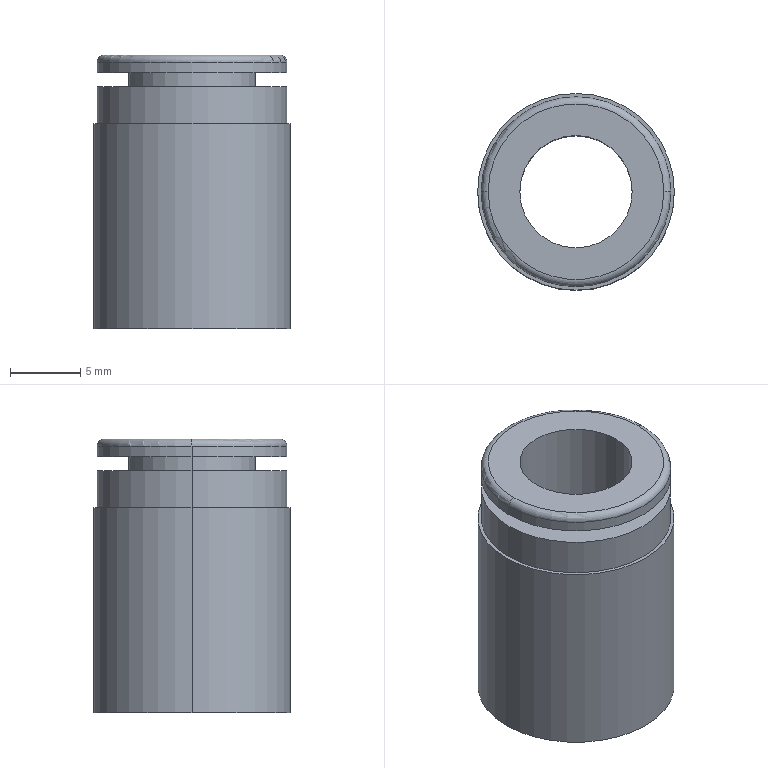Part | STEP file | SS5V1-16S3AD-08B-N1_SV Fittings | 1 solid | 17 faces | box 14 x 14 x 19.5 mm | volume 1887 mm3 | cylinder 10 | plane 5 | torus 2 | commonest cylinder face diameters 13.5 x4 8 x2 9 x2 14 x2
STEP:
#1=CARTESIAN_POINT('',(0.,0.,0.));
#2=DIRECTION('',(0.,0.,1.));
#3=DIRECTION('',(1.,0.,0.));
#4=AXIS2_PLACEMENT_3D('',#1,#2,#3);
#5=CARTESIAN_POINT('',(-6.75,0.,19.));
#6=VERTEX_POINT('',#5);
#7=CARTESIAN_POINT('',(6.75,0.,19.));
#8=VERTEX_POINT('',#7);
#9=CARTESIAN_POINT('',(0.,0.,19.));
#10=DIRECTION('',(0.,0.,-1.));
#11=DIRECTION('',(1.,0.,0.));
#12=AXIS2_PLACEMENT_3D('',#9,#10,#11);
#13=CIRCLE('',#12,6.75);
#14=CARTESIAN_POINT('',(0.,0.,19.));
#15=DIRECTION('',(0.,0.,1.));
#16=DIRECTION('',(1.,0.,0.));
#17=AXIS2_PLACEMENT_3D('',#14,#15,#16);
#18=TOROIDAL_SURFACE('',#17,6.25,0.5);
#19=CARTESIAN_POINT('',(6.283,0.));
#20=DIRECTION('',(-1.,0.));
#21=VECTOR('',#20,1.);
#22=LINE('',#19,#21);
#23=(GEOMETRIC_REPRESENTATION_CONTEXT(2)PARAMETRIC_REPRESENTATION_CONTEXT()REPRESENTATION_CONTEXT('',''));
#24=DEFINITIONAL_REPRESENTATION('',(#22),#23);
#25=PCURVE('',#18,#24);
#26=CARTESIAN_POINT('',(0.,0.,19.5));
#27=DIRECTION('',(0.,0.,-1.));
#28=DIRECTION('',(-1.,0.,0.));
#29=AXIS2_PLACEMENT_3D('',#26,#27,#28);
#30=CYLINDRICAL_SURFACE('',#29,6.75);
#31=CARTESIAN_POINT('',(-3.142,0.5));
#32=DIRECTION('',(1.,0.));
#33=VECTOR('',#32,1.);
#34=LINE('',#31,#33);
#35=(GEOMETRIC_REPRESENTATION_CONTEXT(2)PARAMETRIC_REPRESENTATION_CONTEXT()REPRESENTATION_CONTEXT('',''));
#36=DEFINITIONAL_REPRESENTATION('',(#34),#35);
#37=PCURVE('',#30,#36);
#38=SURFACE_CURVE('',#13,(#25,#37),.PCURVE_S1.);
#39=EDGE_CURVE('',#6,#8,#38,.T.);
#40=ORIENTED_EDGE('',*,*,#39,.F.);
#41=CARTESIAN_POINT('',(-6.25,0.,19.5));
#42=VERTEX_POINT('',#41);
#43=CARTESIAN_POINT('',(-6.25,0.,19.));
#44=DIRECTION('',(0.,1.,0.));
#45=DIRECTION('',(-1.,0.,0.));
#46=AXIS2_PLACEMENT_3D('',#43,#44,#45);
#47=CIRCLE('',#46,0.5);
#48=CARTESIAN_POINT('',(3.142,0.));
#49=DIRECTION('',(0.,1.));
#50=VECTOR('',#49,1.);
#51=LINE('',#48,#50);
#52=(GEOMETRIC_REPRESENTATION_CONTEXT(2)PARAMETRIC_REPRESENTATION_CONTEXT()REPRESENTATION_CONTEXT('',''));
#53=DEFINITIONAL_REPRESENTATION('',(#51),#52);
#54=PCURVE('',#18,#53);
#55=CARTESIAN_POINT('',(0.,0.,19.));
#56=DIRECTION('',(0.,0.,1.));
#57=DIRECTION('',(1.,0.,0.));
#58=AXIS2_PLACEMENT_3D('',#55,#56,#57);
#59=TOROIDAL_SURFACE('',#58,6.25,0.5);
#60=CARTESIAN_POINT('',(3.142,0.));
#61=DIRECTION('',(0.,1.));
#62=VECTOR('',#61,1.);
#63=LINE('',#60,#62);
#64=(GEOMETRIC_REPRESENTATION_CONTEXT(2)PARAMETRIC_REPRESENTATION_CONTEXT()REPRESENTATION_CONTEXT('',''));
#65=DEFINITIONAL_REPRESENTATION('',(#63),#64);
#66=PCURVE('',#59,#65);
#67=SURFACE_CURVE('',#47,(#54,#66),.PCURVE_S1.);
#68=EDGE_CURVE('',#6,#42,#67,.T.);
#69=ORIENTED_EDGE('',*,*,#68,.T.);
#70=CARTESIAN_POINT('',(6.25,0.,19.5));
#71=VERTEX_POINT('',#70);
#72=CARTESIAN_POINT('',(0.,0.,19.5));
#73=DIRECTION('',(0.,0.,1.));
#74=DIRECTION('',(1.,0.,0.));
#75=AXIS2_PLACEMENT_3D('',#72,#73,#74);
#76=CIRCLE('',#75,6.25);
#77=CARTESIAN_POINT('',(0.,1.571));
#78=DIRECTION('',(1.,0.));
#79=VECTOR('',#78,1.);
#80=LINE('',#77,#79);
#81=(GEOMETRIC_REPRESENTATION_CONTEXT(2)PARAMETRIC_REPRESENTATION_CONTEXT()REPRESENTATION_CONTEXT('',''));
#82=DEFINITIONAL_REPRESENTATION('',(#80),#81);
#83=PCURVE('',#18,#82);
#84=CARTESIAN_POINT('',(0.,0.,19.5));
#85=DIRECTION('',(0.,0.,1.));
#86=DIRECTION('',(1.,0.,0.));
#87=AXIS2_PLACEMENT_3D('',#84,#85,#86);
#88=PLANE('',#87);
#89=CARTESIAN_POINT('',(0.,0.));
#90=DIRECTION('',(1.,0.));
#91=AXIS2_PLACEMENT_2D('',#89,#90);
#92=CIRCLE('',#91,6.25);
#93=(GEOMETRIC_REPRESENTATION_CONTEXT(2)PARAMETRIC_REPRESENTATION_CONTEXT()REPRESENTATION_CONTEXT('',''));
#94=DEFINITIONAL_REPRESENTATION('',(#92),#93);
#95=PCURVE('',#88,#94);
#96=SURFACE_CURVE('',#76,(#83,#95),.PCURVE_S1.);
#97=EDGE_CURVE('',#71,#42,#96,.T.);
#98=ORIENTED_EDGE('',*,*,#97,.F.);
#99=CARTESIAN_POINT('',(6.25,0.,19.));
#100=DIRECTION('',(0.,-1.,0.));
#101=DIRECTION('',(0.,0.,-1.));
#102=AXIS2_PLACEMENT_3D('',#99,#100,#101);
#103=CIRCLE('',#102,0.5);
#104=CARTESIAN_POINT('',(0.,-1.571));
#105=DIRECTION('',(0.,1.));
#106=VECTOR('',#105,1.);
#107=LINE('',#104,#106);
#108=(GEOMETRIC_REPRESENTATION_CONTEXT(2)PARAMETRIC_REPRESENTATION_CONTEXT()REPRESENTATION_CONTEXT('',''));
#109=DEFINITIONAL_REPRESENTATION('',(#107),#108);
#110=PCURVE('',#18,#109);
#111=CARTESIAN_POINT('',(6.283,-1.571));
#112=DIRECTION('',(0.,1.));
#113=VECTOR('',#112,1.);
#114=LINE('',#111,#113);
#115=(GEOMETRIC_REPRESENTATION_CONTEXT(2)PARAMETRIC_REPRESENTATION_CONTEXT()REPRESENTATION_CONTEXT('',''));
#116=DEFINITIONAL_REPRESENTATION('',(#114),#115);
#117=PCURVE('',#59,#116);
#118=SURFACE_CURVE('',#103,(#110,#117),.PCURVE_S1.);
#119=EDGE_CURVE('',#8,#71,#118,.T.);
#120=ORIENTED_EDGE('',*,*,#119,.F.);
#121=EDGE_LOOP('',(#40,#69,#98,#120));
#122=FACE_BOUND('',#121,.T.);
#123=ADVANCED_FACE('',(#122),#18,.T.);
#124=ORIENTED_EDGE('',*,*,#39,.T.);
#125=CARTESIAN_POINT('',(6.75,0.,18.25));
#126=VERTEX_POINT('',#125);
#127=CARTESIAN_POINT('',(6.75,0.,19.5));
#128=DIRECTION('',(0.,0.,-1.));
#129=VECTOR('',#128,1.);
#130=LINE('',#127,#129);
#131=CARTESIAN_POINT('',(3.142,0.));
#132=DIRECTION('',(0.,1.));
#133=VECTOR('',#132,1.);
#134=LINE('',#131,#133);
#135=(GEOMETRIC_REPRESENTATION_CONTEXT(2)PARAMETRIC_REPRESENTATION_CONTEXT()REPRESENTATION_CONTEXT('',''));
#136=DEFINITIONAL_REPRESENTATION('',(#134),#135);
#137=PCURVE('',#30,#136);
#138=CARTESIAN_POINT('',(0.,0.,19.5));
#139=DIRECTION('',(0.,0.,-1.));
#140=DIRECTION('',(-1.,0.,0.));
#141=AXIS2_PLACEMENT_3D('',#138,#139,#140);
#142=CYLINDRICAL_SURFACE('',#141,6.75);
#143=CARTESIAN_POINT('',(3.142,0.));
#144=DIRECTION('',(0.,1.));
#145=VECTOR('',#144,1.);
#146=LINE('',#143,#145);
#147=(GEOMETRIC_REPRESENTATION_CONTEXT(2)PARAMETRIC_REPRESENTATION_CONTEXT()REPRESENTATION_CONTEXT('',''));
#148=DEFINITIONAL_REPRESENTATION('',(#146),#147);
#149=PCURVE('',#142,#148);
#150=SURFACE_CURVE('',#130,(#137,#149),.PCURVE_S1.);
#151=EDGE_CURVE('',#8,#126,#150,.T.);
#152=ORIENTED_EDGE('',*,*,#151,.T.);
#153=CARTESIAN_POINT('',(-6.75,0.,18.25));
#154=VERTEX_POINT('',#153);
#155=CARTESIAN_POINT('',(0.,0.,18.25));
#156=DIRECTION('',(0.,0.,1.));
#157=DIRECTION('',(1.,0.,0.));
#158=AXIS2_PLACEMENT_3D('',#155,#156,#157);
#159=CIRCLE('',#158,6.75);
#160=CARTESIAN_POINT('',(3.142,1.25));
#161=DIRECTION('',(-1.,0.));
#162=VECTOR('',#161,1.);
#163=LINE('',#160,#162);
#164=(GEOMETRIC_REPRESENTATION_CONTEXT(2)PARAMETRIC_REPRESENTATION_CONTEXT()REPRESENTATION_CONTEXT('',''));
#165=DEFINITIONAL_REPRESENTATION('',(#163),#164);
#166=PCURVE('',#30,#165);
#167=CARTESIAN_POINT('',(0.,0.,18.25));
#168=DIRECTION('',(0.,0.,1.));
#169=DIRECTION('',(1.,0.,0.));
#170=AXIS2_PLACEMENT_3D('',#167,#168,#169);
#171=PLANE('',#170);
#172=CARTESIAN_POINT('',(0.,0.));
#173=DIRECTION('',(1.,0.));
#174=AXIS2_PLACEMENT_2D('',#172,#173);
#175=CIRCLE('',#174,6.75);
#176=(GEOMETRIC_REPRESENTATION_CONTEXT(2)PARAMETRIC_REPRESENTATION_CONTEXT()REPRESENTATION_CONTEXT('',''));
#177=DEFINITIONAL_REPRESENTATION('',(#175),#176);
#178=PCURVE('',#171,#177);
#179=SURFACE_CURVE('',#159,(#166,#178),.PCURVE_S1.);
#180=EDGE_CURVE('',#126,#154,#179,.T.);
#181=ORIENTED_EDGE('',*,*,#180,.T.);
#182=CARTESIAN_POINT('',(-6.75,0.,19.5));
#183=DIRECTION('',(0.,0.,-1.));
#184=VECTOR('',#183,1.);
#185=LINE('',#182,#184);
#186=CARTESIAN_POINT('',(0.,0.));
#187=DIRECTION('',(0.,1.));
#188=VECTOR('',#187,1.);
#189=LINE('',#186,#188);
#190=(GEOMETRIC_REPRESENTATION_CONTEXT(2)PARAMETRIC_REPRESENTATION_CONTEXT()REPRESENTATION_CONTEXT('',''));
#191=DEFINITIONAL_REPRESENTATION('',(#189),#190);
#192=PCURVE('',#30,#191);
#193=CARTESIAN_POINT('',(6.283,0.));
#194=DIRECTION('',(0.,1.));
#195=VECTOR('',#194,1.);
#196=LINE('',#193,#195);
#197=(GEOMETRIC_REPRESENTATION_CONTEXT(2)PARAMETRIC_REPRESENTATION_CONTEXT()REPRESENTATION_CONTEXT('',''));
#198=DEFINITIONAL_REPRESENTATION('',(#196),#197);
#199=PCURVE('',#142,#198);
#200=SURFACE_CURVE('',#185,(#192,#199),.PCURVE_S1.);
#201=EDGE_CURVE('',#6,#154,#200,.T.);
#202=ORIENTED_EDGE('',*,*,#201,.F.);
#203=EDGE_LOOP('',(#124,#152,#181,#202));
#204=FACE_BOUND('',#203,.T.);
#205=ADVANCED_FACE('',(#204),#30,.T.);
#206=CARTESIAN_POINT('',(4.5,0.,18.25));
#207=VERTEX_POINT('',#206);
#208=CARTESIAN_POINT('',(-4.5,0.,18.25));
#209=VERTEX_POINT('',#208);
#210=CARTESIAN_POINT('',(0.,0.,18.25));
#211=DIRECTION('',(0.,0.,1.));
#212=DIRECTION('',(1.,0.,0.));
#213=AXIS2_PLACEMENT_3D('',#210,#211,#212);
#214=CIRCLE('',#213,4.5);
#215=CARTESIAN_POINT('',(0.,0.,18.25));
#216=DIRECTION('',(0.,0.,-1.));
#217=DIRECTION('',(-1.,0.,0.));
#218=AXIS2_PLACEMENT_3D('',#215,#216,#217);
#219=CYLINDRICAL_SURFACE('',#218,4.5);
#220=CARTESIAN_POINT('',(3.142,0.));
#221=DIRECTION('',(-1.,0.));
#222=VECTOR('',#221,1.);
#223=LINE('',#220,#222);
#224=(GEOMETRIC_REPRESENTATION_CONTEXT(2)PARAMETRIC_REPRESENTATION_CONTEXT()REPRESENTATION_CONTEXT('',''));
#225=DEFINITIONAL_REPRESENTATION('',(#223),#224);
#226=PCURVE('',#219,#225);
#227=CARTESIAN_POINT('',(0.,0.));
#228=DIRECTION('',(1.,0.));
#229=AXIS2_PLACEMENT_2D('',#227,#228);
#230=CIRCLE('',#229,4.5);
#231=(GEOMETRIC_REPRESENTATION_CONTEXT(2)PARAMETRIC_REPRESENTATION_CONTEXT()REPRESENTATION_CONTEXT('',''));
#232=DEFINITIONAL_REPRESENTATION('',(#230),#231);
#233=PCURVE('',#171,#232);
#234=SURFACE_CURVE('',#214,(#226,#233),.PCURVE_S1.);
#235=EDGE_CURVE('',#207,#209,#234,.T.);
#236=ORIENTED_EDGE('',*,*,#235,.F.);
#237=CARTESIAN_POINT('',(4.5,0.,17.25));
#238=VERTEX_POINT('',#237);
#239=CARTESIAN_POINT('',(4.5,0.,18.25));
#240=DIRECTION('',(0.,0.,-1.));
#241=VECTOR('',#240,1.);
#242=LINE('',#239,#241);
#243=CARTESIAN_POINT('',(3.142,0.));
#244=DIRECTION('',(0.,1.));
#245=VECTOR('',#244,1.);
#246=LINE('',#243,#245);
#247=(GEOMETRIC_REPRESENTATION_CONTEXT(2)PARAMETRIC_REPRESENTATION_CONTEXT()REPRESENTATION_CONTEXT('',''));
#248=DEFINITIONAL_REPRESENTATION('',(#246),#247);
#249=PCURVE('',#219,#248);
#250=CARTESIAN_POINT('',(0.,0.,18.25));
#251=DIRECTION('',(0.,0.,-1.));
#252=DIRECTION('',(-1.,0.,0.));
#253=AXIS2_PLACEMENT_3D('',#250,#251,#252);
#254=CYLINDRICAL_SURFACE('',#253,4.5);
#255=CARTESIAN_POINT('',(3.142,0.));
#256=DIRECTION('',(0.,1.));
#257=VECTOR('',#256,1.);
#258=LINE('',#255,#257);
#259=(GEOMETRIC_REPRESENTATION_CONTEXT(2)PARAMETRIC_REPRESENTATION_CONTEXT()REPRESENTATION_CONTEXT('',''));
#260=DEFINITIONAL_REPRESENTATION('',(#258),#259);
#261=PCURVE('',#254,#260);
#262=SURFACE_CURVE('',#242,(#249,#261),.PCURVE_S1.);
#263=EDGE_CURVE('',#207,#238,#262,.T.);
#264=ORIENTED_EDGE('',*,*,#263,.T.);
#265=CARTESIAN_POINT('',(-4.5,0.,17.25));
#266=VERTEX_POINT('',#265);
#267=CARTESIAN_POINT('',(0.,0.,17.25));
#268=DIRECTION('',(0.,0.,1.));
#269=DIRECTION('',(1.,0.,0.));
#270=AXIS2_PLACEMENT_3D('',#267,#268,#269);
#271=CIRCLE('',#270,4.5);
#272=CARTESIAN_POINT('',(3.142,1.));
#273=DIRECTION('',(-1.,0.));
#274=VECTOR('',#273,1.);
#275=LINE('',#272,#274);
#276=(GEOMETRIC_REPRESENTATION_CONTEXT(2)PARAMETRIC_REPRESENTATION_CONTEXT()REPRESENTATION_CONTEXT('',''));
#277=DEFINITIONAL_REPRESENTATION('',(#275),#276);
#278=PCURVE('',#219,#277);
#279=CARTESIAN_POINT('',(0.,0.,17.25));
#280=DIRECTION('',(0.,0.,1.));
#281=DIRECTION('',(1.,0.,0.));
#282=AXIS2_PLACEMENT_3D('',#279,#280,#281);
#283=PLANE('',#282);
#284=CARTESIAN_POINT('',(0.,0.));
#285=DIRECTION('',(1.,0.));
#286=AXIS2_PLACEMENT_2D('',#284,#285);
#287=CIRCLE('',#286,4.5);
#288=(GEOMETRIC_REPRESENTATION_CONTEXT(2)PARAMETRIC_REPRESENTATION_CONTEXT()REPRESENTATION_CONTEXT('',''));
#289=DEFINITIONAL_REPRESENTATION('',(#287),#288);
#290=PCURVE('',#283,#289);
#291=SURFACE_CURVE('',#271,(#278,#290),.PCURVE_S1.);
#292=EDGE_CURVE('',#238,#266,#291,.T.);
#293=ORIENTED_EDGE('',*,*,#292,.T.);
#294=CARTESIAN_POINT('',(-4.5,0.,18.25));
#295=DIRECTION('',(0.,0.,-1.));
#296=VECTOR('',#295,1.);
#297=LINE('',#294,#296);
#298=CARTESIAN_POINT('',(0.,0.));
#299=DIRECTION('',(0.,1.));
#300=VECTOR('',#299,1.);
#301=LINE('',#298,#300);
#302=(GEOMETRIC_REPRESENTATION_CONTEXT(2)PARAMETRIC_REPRESENTATION_CONTEXT()REPRESENTATION_CONTEXT('',''));
#303=DEFINITIONAL_REPRESENTATION('',(#301),#302);
#304=PCURVE('',#219,#303);
#305=CARTESIAN_POINT('',(6.283,0.));
#306=DIRECTION('',(0.,1.));
#307=VECTOR('',#306,1.);
#308=LINE('',#305,#307);
#309=(GEOMETRIC_REPRESENTATION_CONTEXT(2)PARAMETRIC_REPRESENTATION_CONTEXT()REPRESENTATION_CONTEXT('',''));
#310=DEFINITIONAL_REPRESENTATION('',(#308),#309);
#311=PCURVE('',#254,#310);
#312=SURFACE_CURVE('',#297,(#304,#311),.PCURVE_S1.);
#313=EDGE_CURVE('',#209,#266,#312,.T.);
#314=ORIENTED_EDGE('',*,*,#313,.F.);
#315=EDGE_LOOP('',(#236,#264,#293,#314));
#316=FACE_BOUND('',#315,.T.);
#317=ADVANCED_FACE('',(#316),#219,.T.);
#318=CARTESIAN_POINT('',(6.75,0.,17.25));
#319=VERTEX_POINT('',#318);
#320=CARTESIAN_POINT('',(-6.75,0.,17.25));
#321=VERTEX_POINT('',#320);
#322=CARTESIAN_POINT('',(0.,0.,17.25));
#323=DIRECTION('',(0.,0.,1.));
#324=DIRECTION('',(1.,0.,0.));
#325=AXIS2_PLACEMENT_3D('',#322,#323,#324);
#326=CIRCLE('',#325,6.75);
#327=CARTESIAN_POINT('',(0.,0.,17.25));
#328=DIRECTION('',(0.,0.,-1.));
#329=DIRECTION('',(-1.,0.,0.));
#330=AXIS2_PLACEMENT_3D('',#327,#328,#329);
#331=CYLINDRICAL_SURFACE('',#330,6.75);
#332=CARTESIAN_POINT('',(3.142,0.));
#333=DIRECTION('',(-1.,0.));
#334=VECTOR('',#333,1.);
#335=LINE('',#332,#334);
#336=(GEOMETRIC_REPRESENTATION_CONTEXT(2)PARAMETRIC_REPRESENTATION_CONTEXT()REPRESENTATION_CONTEXT('',''));
#337=DEFINITIONAL_REPRESENTATION('',(#335),#336);
#338=PCURVE('',#331,#337);
#339=CARTESIAN_POINT('',(0.,0.));
#340=DIRECTION('',(1.,0.));
#341=AXIS2_PLACEMENT_2D('',#339,#340);
#342=CIRCLE('',#341,6.75);
#343=(GEOMETRIC_REPRESENTATION_CONTEXT(2)PARAMETRIC_REPRESENTATION_CONTEXT()REPRESENTATION_CONTEXT('',''));
#344=DEFINITIONAL_REPRESENTATION('',(#342),#343);
#345=PCURVE('',#283,#344);
#346=SURFACE_CURVE('',#326,(#338,#345),.PCURVE_S1.);
#347=EDGE_CURVE('',#319,#321,#346,.T.);
#348=ORIENTED_EDGE('',*,*,#347,.F.);
#349=CARTESIAN_POINT('',(6.75,0.,14.6));
#350=VERTEX_POINT('',#349);
#351=CARTESIAN_POINT('',(6.75,0.,17.25));
#352=DIRECTION('',(0.,0.,-1.));
#353=VECTOR('',#352,1.);
#354=LINE('',#351,#353);
#355=CARTESIAN_POINT('',(3.142,0.));
#356=DIRECTION('',(0.,1.));
#357=VECTOR('',#356,1.);
#358=LINE('',#355,#357);
#359=(GEOMETRIC_REPRESENTATION_CONTEXT(2)PARAMETRIC_REPRESENTATION_CONTEXT()REPRESENTATION_CONTEXT('',''));
#360=DEFINITIONAL_REPRESENTATION('',(#358),#359);
#361=PCURVE('',#331,#360);
#362=CARTESIAN_POINT('',(0.,0.,17.25));
#363=DIRECTION('',(0.,0.,-1.));
#364=DIRECTION('',(-1.,0.,0.));
#365=AXIS2_PLACEMENT_3D('',#362,#363,#364);
#366=CYLINDRICAL_SURFACE('',#365,6.75);
#367=CARTESIAN_POINT('',(3.142,0.));
#368=DIRECTION('',(0.,1.));
#369=VECTOR('',#368,1.);
#370=LINE('',#367,#369);
#371=(GEOMETRIC_REPRESENTATION_CONTEXT(2)PARAMETRIC_REPRESENTATION_CONTEXT()REPRESENTATION_CONTEXT('',''));
#372=DEFINITIONAL_REPRESENTATION('',(#370),#371);
#373=PCURVE('',#366,#372);
#374=SURFACE_CURVE('',#354,(#361,#373),.PCURVE_S1.);
#375=EDGE_CURVE('',#319,#350,#374,.T.);
#376=ORIENTED_EDGE('',*,*,#375,.T.);
#377=CARTESIAN_POINT('',(-6.75,0.,14.6));
#378=VERTEX_POINT('',#377);
#379=CARTESIAN_POINT('',(0.,0.,14.6));
#380=DIRECTION('',(0.,0.,1.));
#381=DIRECTION('',(1.,0.,0.));
#382=AXIS2_PLACEMENT_3D('',#379,#380,#381);
#383=CIRCLE('',#382,6.75);
#384=CARTESIAN_POINT('',(3.142,2.65));
#385=DIRECTION('',(-1.,0.));
#386=VECTOR('',#385,1.);
#387=LINE('',#384,#386);
#388=(GEOMETRIC_REPRESENTATION_CONTEXT(2)PARAMETRIC_REPRESENTATION_CONTEXT()REPRESENTATION_CONTEXT('',''));
#389=DEFINITIONAL_REPRESENTATION('',(#387),#388);
#390=PCURVE('',#331,#389);
#391=CARTESIAN_POINT('',(0.,0.,14.6));
#392=DIRECTION('',(0.,0.,1.));
#393=DIRECTION('',(1.,0.,0.));
#394=AXIS2_PLACEMENT_3D('',#391,#392,#393);
#395=PLANE('',#394);
#396=CARTESIAN_POINT('',(0.,0.));
#397=DIRECTION('',(1.,0.));
#398=AXIS2_PLACEMENT_2D('',#396,#397);
#399=CIRCLE('',#398,6.75);
#400=(GEOMETRIC_REPRESENTATION_CONTEXT(2)PARAMETRIC_REPRESENTATION_CONTEXT()REPRESENTATION_CONTEXT('',''));
#401=DEFINITIONAL_REPRESENTATION('',(#399),#400);
#402=PCURVE('',#395,#401);
#403=SURFACE_CURVE('',#383,(#390,#402),.PCURVE_S1.);
#404=EDGE_CURVE('',#350,#378,#403,.T.);
#405=ORIENTED_EDGE('',*,*,#404,.T.);
#406=CARTESIAN_POINT('',(-6.75,0.,17.25));
#407=DIRECTION('',(0.,0.,-1.));
#408=VECTOR('',#407,1.);
#409=LINE('',#406,#408);
#410=CARTESIAN_POINT('',(0.,0.));
#411=DIRECTION('',(0.,1.));
#412=VECTOR('',#411,1.);
#413=LINE('',#410,#412);
#414=(GEOMETRIC_REPRESENTATION_CONTEXT(2)PARAMETRIC_REPRESENTATION_CONTEXT()REPRESENTATION_CONTEXT('',''));
#415=DEFINITIONAL_REPRESENTATION('',(#413),#414);
#416=PCURVE('',#331,#415);
#417=CARTESIAN_POINT('',(6.283,0.));
#418=DIRECTION('',(0.,1.));
#419=VECTOR('',#418,1.);
#420=LINE('',#417,#419);
#421=(GEOMETRIC_REPRESENTATION_CONTEXT(2)PARAMETRIC_REPRESENTATION_CONTEXT()REPRESENTATION_CONTEXT('',''));
#422=DEFINITIONAL_REPRESENTATION('',(#420),#421);
#423=PCURVE('',#366,#422);
#424=SURFACE_CURVE('',#409,(#416,#423),.PCURVE_S1.);
#425=EDGE_CURVE('',#321,#378,#424,.T.);
#426=ORIENTED_EDGE('',*,*,#425,.F.);
#427=EDGE_LOOP('',(#348,#376,#405,#426));
#428=FACE_BOUND('',#427,.T.);
#429=ADVANCED_FACE('',(#428),#331,.T.);
#430=CARTESIAN_POINT('',(-4.,0.,19.5));
#431=VERTEX_POINT('',#430);
#432=CARTESIAN_POINT('',(-4.,0.,0.));
#433=VERTEX_POINT('',#432);
#434=CARTESIAN_POINT('',(-4.,0.,14.6));
#435=DIRECTION('',(0.,0.,-1.));
#436=VECTOR('',#435,1.);
#437=LINE('',#434,#436);
#438=CARTESIAN_POINT('',(0.,0.,14.6));
#439=DIRECTION('',(0.,0.,-1.));
#440=DIRECTION('',(-1.,0.,0.));
#441=AXIS2_PLACEMENT_3D('',#438,#439,#440);
#442=CYLINDRICAL_SURFACE('',#441,4.);
#443=CARTESIAN_POINT('',(6.283,0.));
#444=DIRECTION('',(0.,1.));
#445=VECTOR('',#444,1.);
#446=LINE('',#443,#445);
#447=(GEOMETRIC_REPRESENTATION_CONTEXT(2)PARAMETRIC_REPRESENTATION_CONTEXT()REPRESENTATION_CONTEXT('',''));
#448=DEFINITIONAL_REPRESENTATION('',(#446),#447);
#449=PCURVE('',#442,#448);
#450=CARTESIAN_POINT('',(0.,0.,14.6));
#451=DIRECTION('',(0.,0.,-1.));
#452=DIRECTION('',(-1.,0.,0.));
#453=AXIS2_PLACEMENT_3D('',#450,#451,#452);
#454=CYLINDRICAL_SURFACE('',#453,4.);
#455=CARTESIAN_POINT('',(0.,0.));
#456=DIRECTION('',(0.,1.));
#457=VECTOR('',#456,1.);
#458=LINE('',#455,#457);
#459=(GEOMETRIC_REPRESENTATION_CONTEXT(2)PARAMETRIC_REPRESENTATION_CONTEXT()REPRESENTATION_CONTEXT('',''));
#460=DEFINITIONAL_REPRESENTATION('',(#458),#459);
#461=PCURVE('',#454,#460);
#462=SURFACE_CURVE('',#437,(#449,#461),.PCURVE_S1.);
#463=EDGE_CURVE('',#431,#433,#462,.T.);
#464=ORIENTED_EDGE('',*,*,#463,.T.);
#465=CARTESIAN_POINT('',(4.,0.,0.));
#466=VERTEX_POINT('',#465);
#467=CARTESIAN_POINT('',(0.,0.,0.));
#468=DIRECTION('',(0.,0.,1.));
#469=DIRECTION('',(1.,0.,0.));
#470=AXIS2_PLACEMENT_3D('',#467,#468,#469);
#471=CIRCLE('',#470,4.);
#472=CARTESIAN_POINT('',(9.425,14.6));
#473=DIRECTION('',(-1.,0.));
#474=VECTOR('',#473,1.);
#475=LINE('',#472,#474);
#476=(GEOMETRIC_REPRESENTATION_CONTEXT(2)PARAMETRIC_REPRESENTATION_CONTEXT()REPRESENTATION_CONTEXT('',''));
#477=DEFINITIONAL_REPRESENTATION('',(#475),#476);
#478=PCURVE('',#442,#477);
#479=CARTESIAN_POINT('',(0.,0.,0.));
#480=DIRECTION('',(0.,0.,1.));
#481=DIRECTION('',(1.,0.,0.));
#482=AXIS2_PLACEMENT_3D('',#479,#480,#481);
#483=PLANE('',#482);
#484=CARTESIAN_POINT('',(0.,0.));
#485=DIRECTION('',(1.,0.));
#486=AXIS2_PLACEMENT_2D('',#484,#485);
#487=CIRCLE('',#486,4.);
#488=(GEOMETRIC_REPRESENTATION_CONTEXT(2)PARAMETRIC_REPRESENTATION_CONTEXT()REPRESENTATION_CONTEXT('',''));
#489=DEFINITIONAL_REPRESENTATION('',(#487),#488);
#490=PCURVE('',#483,#489);
#491=SURFACE_CURVE('',#471,(#478,#490),.PCURVE_S1.);
#492=EDGE_CURVE('',#433,#466,#491,.T.);
#493=ORIENTED_EDGE('',*,*,#492,.T.);
#494=CARTESIAN_POINT('',(4.,0.,19.5));
#495=VERTEX_POINT('',#494);
#496=CARTESIAN_POINT('',(4.,0.,14.6));
#497=DIRECTION('',(0.,0.,-1.));
#498=VECTOR('',#497,1.);
#499=LINE('',#496,#498);
#500=CARTESIAN_POINT('',(3.142,0.));
#501=DIRECTION('',(0.,1.));
#502=VECTOR('',#501,1.);
#503=LINE('',#500,#502);
#504=(GEOMETRIC_REPRESENTATION_CONTEXT(2)PARAMETRIC_REPRESENTATION_CONTEXT()REPRESENTATION_CONTEXT('',''));
#505=DEFINITIONAL_REPRESENTATION('',(#503),#504);
#506=PCURVE('',#442,#505);
#507=CARTESIAN_POINT('',(3.142,0.));
#508=DIRECTION('',(0.,1.));
#509=VECTOR('',#508,1.);
#510=LINE('',#507,#509);
#511=(GEOMETRIC_REPRESENTATION_CONTEXT(2)PARAMETRIC_REPRESENTATION_CONTEXT()REPRESENTATION_CONTEXT('',''));
#512=DEFINITIONAL_REPRESENTATION('',(#510),#511);
#513=PCURVE('',#454,#512);
#514=SURFACE_CURVE('',#499,(#506,#513),.PCURVE_S1.);
#515=EDGE_CURVE('',#495,#466,#514,.T.);
#516=ORIENTED_EDGE('',*,*,#515,.F.);
#517=CARTESIAN_POINT('',(0.,0.,19.5));
#518=DIRECTION('',(0.,0.,1.));
#519=DIRECTION('',(1.,0.,0.));
#520=AXIS2_PLACEMENT_3D('',#517,#518,#519);
#521=CIRCLE('',#520,4.);
#522=CARTESIAN_POINT('',(9.425,-4.9));
#523=DIRECTION('',(-1.,0.));
#524=VECTOR('',#523,1.);
#525=LINE('',#522,#524);
#526=(GEOMETRIC_REPRESENTATION_CONTEXT(2)PARAMETRIC_REPRESENTATION_CONTEXT()REPRESENTATION_CONTEXT('',''));
#527=DEFINITIONAL_REPRESENTATION('',(#525),#526);
#528=PCURVE('',#442,#527);
#529=CARTESIAN_POINT('',(0.,0.));
#530=DIRECTION('',(1.,0.));
#531=AXIS2_PLACEMENT_2D('',#529,#530);
#532=CIRCLE('',#531,4.);
#533=(GEOMETRIC_REPRESENTATION_CONTEXT(2)PARAMETRIC_REPRESENTATION_CONTEXT()REPRESENTATION_CONTEXT('',''));
#534=DEFINITIONAL_REPRESENTATION('',(#532),#533);
#535=PCURVE('',#88,#534);
#536=SURFACE_CURVE('',#521,(#528,#535),.PCURVE_S1.);
#537=EDGE_CURVE('',#431,#495,#536,.T.);
#538=ORIENTED_EDGE('',*,*,#537,.F.);
#539=EDGE_LOOP('',(#464,#493,#516,#538));
#540=FACE_BOUND('',#539,.F.);
#541=ADVANCED_FACE('',(#540),#442,.F.);
#542=CARTESIAN_POINT('',(7.,0.,14.6));
#543=VERTEX_POINT('',#542);
#544=CARTESIAN_POINT('',(-7.,0.,14.6));
#545=VERTEX_POINT('',#544);
#546=CARTESIAN_POINT('',(0.,0.,14.6));
#547=DIRECTION('',(0.,0.,1.));
#548=DIRECTION('',(1.,0.,0.));
#549=AXIS2_PLACEMENT_3D('',#546,#547,#548);
#550=CIRCLE('',#549,7.);
#551=CARTESIAN_POINT('',(0.,0.,14.6));
#552=DIRECTION('',(0.,0.,-1.));
#553=DIRECTION('',(-1.,0.,0.));
#554=AXIS2_PLACEMENT_3D('',#551,#552,#553);
#555=CYLINDRICAL_SURFACE('',#554,7.);
#556=CARTESIAN_POINT('',(3.142,0.));
#557=DIRECTION('',(-1.,0.));
#558=VECTOR('',#557,1.);
#559=LINE('',#556,#558);
#560=(GEOMETRIC_REPRESENTATION_CONTEXT(2)PARAMETRIC_REPRESENTATION_CONTEXT()REPRESENTATION_CONTEXT('',''));
#561=DEFINITIONAL_REPRESENTATION('',(#559),#560);
#562=PCURVE('',#555,#561);
#563=CARTESIAN_POINT('',(0.,0.));
#564=DIRECTION('',(1.,0.));
#565=AXIS2_PLACEMENT_2D('',#563,#564);
#566=CIRCLE('',#565,7.);
#567=(GEOMETRIC_REPRESENTATION_CONTEXT(2)PARAMETRIC_REPRESENTATION_CONTEXT()REPRESENTATION_CONTEXT('',''));
#568=DEFINITIONAL_REPRESENTATION('',(#566),#567);
#569=PCURVE('',#395,#568);
#570=SURFACE_CURVE('',#550,(#562,#569),.PCURVE_S1.);
#571=EDGE_CURVE('',#543,#545,#570,.T.);
#572=ORIENTED_EDGE('',*,*,#571,.F.);
#573=CARTESIAN_POINT('',(7.,0.,0.));
#574=VERTEX_POINT('',#573);
#575=CARTESIAN_POINT('',(7.,0.,14.6));
#576=DIRECTION('',(0.,0.,-1.));
#577=VECTOR('',#576,1.);
#578=LINE('',#575,#577);
#579=CARTESIAN_POINT('',(3.142,0.));
#580=DIRECTION('',(0.,1.));
#581=VECTOR('',#580,1.);
#582=LINE('',#579,#581);
#583=(GEOMETRIC_REPRESENTATION_CONTEXT(2)PARAMETRIC_REPRESENTATION_CONTEXT()REPRESENTATION_CONTEXT('',''));
#584=DEFINITIONAL_REPRESENTATION('',(#582),#583);
#585=PCURVE('',#555,#584);
#586=CARTESIAN_POINT('',(0.,0.,14.6));
#587=DIRECTION('',(0.,0.,-1.));
#588=DIRECTION('',(-1.,0.,0.));
#589=AXIS2_PLACEMENT_3D('',#586,#587,#588);
#590=CYLINDRICAL_SURFACE('',#589,7.);
#591=CARTESIAN_POINT('',(3.142,0.));
#592=DIRECTION('',(0.,1.));
#593=VECTOR('',#592,1.);
#594=LINE('',#591,#593);
#595=(GEOMETRIC_REPRESENTATION_CONTEXT(2)PARAMETRIC_REPRESENTATION_CONTEXT()REPRESENTATION_CONTEXT('',''));
#596=DEFINITIONAL_REPRESENTATION('',(#594),#595);
#597=PCURVE('',#590,#596);
#598=SURFACE_CURVE('',#578,(#585,#597),.PCURVE_S1.);
#599=EDGE_CURVE('',#543,#574,#598,.T.);
#600=ORIENTED_EDGE('',*,*,#599,.T.);
#601=CARTESIAN_POINT('',(-7.,0.,0.));
#602=VERTEX_POINT('',#601);
#603=CARTESIAN_POINT('',(0.,0.,0.));
#604=DIRECTION('',(0.,0.,1.));
#605=DIRECTION('',(1.,0.,0.));
#606=AXIS2_PLACEMENT_3D('',#603,#604,#605);
#607=CIRCLE('',#606,7.);
#608=CARTESIAN_POINT('',(3.142,14.6));
#609=DIRECTION('',(-1.,0.));
#610=VECTOR('',#609,1.);
#611=LINE('',#608,#610);
#612=(GEOMETRIC_REPRESENTATION_CONTEXT(2)PARAMETRIC_REPRESENTATION_CONTEXT()REPRESENTATION_CONTEXT('',''));
#613=DEFINITIONAL_REPRESENTATION('',(#611),#612);
#614=PCURVE('',#555,#613);
#615=CARTESIAN_POINT('',(0.,0.));
#616=DIRECTION('',(1.,0.));
#617=AXIS2_PLACEMENT_2D('',#615,#616);
#618=CIRCLE('',#617,7.);
#619=(GEOMETRIC_REPRESENTATION_CONTEXT(2)PARAMETRIC_REPRESENTATION_CONTEXT()REPRESENTATION_CONTEXT('',''));
#620=DEFINITIONAL_REPRESENTATION('',(#618),#619);
#621=PCURVE('',#483,#620);
#622=SURFACE_CURVE('',#607,(#614,#621),.PCURVE_S1.);
#623=EDGE_CURVE('',#574,#602,#622,.T.);
#624=ORIENTED_EDGE('',*,*,#623,.T.);
#625=CARTESIAN_POINT('',(-7.,0.,14.6));
#626=DIRECTION('',(0.,0.,-1.));
#627=VECTOR('',#626,1.);
#628=LINE('',#625,#627);
#629=CARTESIAN_POINT('',(0.,0.));
#630=DIRECTION('',(0.,1.));
#631=VECTOR('',#630,1.);
#632=LINE('',#629,#631);
#633=(GEOMETRIC_REPRESENTATION_CONTEXT(2)PARAMETRIC_REPRESENTATION_CONTEXT()REPRESENTATION_CONTEXT('',''));
#634=DEFINITIONAL_REPRESENTATION('',(#632),#633);
#635=PCURVE('',#555,#634);
#636=CARTESIAN_POINT('',(6.283,0.));
#637=DIRECTION('',(0.,1.));
#638=VECTOR('',#637,1.);
#639=LINE('',#636,#638);
#640=(GEOMETRIC_REPRESENTATION_CONTEXT(2)PARAMETRIC_REPRESENTATION_CONTEXT()REPRESENTATION_CONTEXT('',''));
#641=DEFINITIONAL_REPRESENTATION('',(#639),#640);
#642=PCURVE('',#590,#641);
#643=SURFACE_CURVE('',#628,(#635,#642),.PCURVE_S1.);
#644=EDGE_CURVE('',#545,#602,#643,.T.);
#645=ORIENTED_EDGE('',*,*,#644,.F.);
#646=EDGE_LOOP('',(#572,#600,#624,#645));
#647=FACE_BOUND('',#646,.T.);
#648=ADVANCED_FACE('',(#647),#555,.T.);
#649=CARTESIAN_POINT('',(0.,0.,17.25));
#650=DIRECTION('',(0.,0.,1.));
#651=DIRECTION('',(1.,0.,0.));
#652=AXIS2_PLACEMENT_3D('',#649,#650,#651);
#653=CIRCLE('',#652,6.75);
#654=CARTESIAN_POINT('',(0.,0.));
#655=DIRECTION('',(1.,0.));
#656=AXIS2_PLACEMENT_2D('',#654,#655);
#657=CIRCLE('',#656,6.75);
#658=(GEOMETRIC_REPRESENTATION_CONTEXT(2)PARAMETRIC_REPRESENTATION_CONTEXT()REPRESENTATION_CONTEXT('',''));
#659=DEFINITIONAL_REPRESENTATION('',(#657),#658);
#660=PCURVE('',#283,#659);
#661=CARTESIAN_POINT('',(9.425,0.));
#662=DIRECTION('',(-1.,0.));
#663=VECTOR('',#662,1.);
#664=LINE('',#661,#663);
#665=(GEOMETRIC_REPRESENTATION_CONTEXT(2)PARAMETRIC_REPRESENTATION_CONTEXT()REPRESENTATION_CONTEXT('',''));
#666=DEFINITIONAL_REPRESENTATION('',(#664),#665);
#667=PCURVE('',#366,#666);
#668=SURFACE_CURVE('',#653,(#660,#667),.PCURVE_S1.);
#669=EDGE_CURVE('',#321,#319,#668,.T.);
#670=ORIENTED_EDGE('',*,*,#669,.T.);
#671=ORIENTED_EDGE('',*,*,#347,.T.);
#672=EDGE_LOOP('',(#670,#671));
#673=FACE_BOUND('',#672,.T.);
#674=CARTESIAN_POINT('',(0.,0.,17.25));
#675=DIRECTION('',(0.,0.,1.));
#676=DIRECTION('',(1.,0.,0.));
#677=AXIS2_PLACEMENT_3D('',#674,#675,#676);
#678=CIRCLE('',#677,4.5);
#679=CARTESIAN_POINT('',(0.,0.));
#680=DIRECTION('',(1.,0.));
#681=AXIS2_PLACEMENT_2D('',#679,#680);
#682=CIRCLE('',#681,4.5);
#683=(GEOMETRIC_REPRESENTATION_CONTEXT(2)PARAMETRIC_REPRESENTATION_CONTEXT()REPRESENTATION_CONTEXT('',''));
#684=DEFINITIONAL_REPRESENTATION('',(#682),#683);
#685=PCURVE('',#283,#684);
#686=CARTESIAN_POINT('',(9.425,1.));
#687=DIRECTION('',(-1.,0.));
#688=VECTOR('',#687,1.);
#689=LINE('',#686,#688);
#690=(GEOMETRIC_REPRESENTATION_CONTEXT(2)PARAMETRIC_REPRESENTATION_CONTEXT()REPRESENTATION_CONTEXT('',''));
#691=DEFINITIONAL_REPRESENTATION('',(#689),#690);
#692=PCURVE('',#254,#691);
#693=SURFACE_CURVE('',#678,(#685,#692),.PCURVE_S1.);
#694=EDGE_CURVE('',#266,#238,#693,.T.);
#695=ORIENTED_EDGE('',*,*,#694,.F.);
#696=ORIENTED_EDGE('',*,*,#292,.F.);
#697=EDGE_LOOP('',(#695,#696));
#698=FACE_BOUND('',#697,.T.);
#699=ADVANCED_FACE('',(#673,#698),#283,.T.);
#700=CARTESIAN_POINT('',(0.,0.,14.6));
#701=DIRECTION('',(0.,0.,1.));
#702=DIRECTION('',(1.,0.,0.));
#703=AXIS2_PLACEMENT_3D('',#700,#701,#702);
#704=CIRCLE('',#703,7.);
#705=CARTESIAN_POINT('',(0.,0.));
#706=DIRECTION('',(1.,0.));
#707=AXIS2_PLACEMENT_2D('',#705,#706);
#708=CIRCLE('',#707,7.);
#709=(GEOMETRIC_REPRESENTATION_CONTEXT(2)PARAMETRIC_REPRESENTATION_CONTEXT()REPRESENTATION_CONTEXT('',''));
#710=DEFINITIONAL_REPRESENTATION('',(#708),#709);
#711=PCURVE('',#395,#710);
#712=CARTESIAN_POINT('',(9.425,0.));
#713=DIRECTION('',(-1.,0.));
#714=VECTOR('',#713,1.);
#715=LINE('',#712,#714);
#716=(GEOMETRIC_REPRESENTATION_CONTEXT(2)PARAMETRIC_REPRESENTATION_CONTEXT()REPRESENTATION_CONTEXT('',''));
#717=DEFINITIONAL_REPRESENTATION('',(#715),#716);
#718=PCURVE('',#590,#717);
#719=SURFACE_CURVE('',#704,(#711,#718),.PCURVE_S1.);
#720=EDGE_CURVE('',#545,#543,#719,.T.);
#721=ORIENTED_EDGE('',*,*,#720,.T.);
#722=ORIENTED_EDGE('',*,*,#571,.T.);
#723=EDGE_LOOP('',(#721,#722));
#724=FACE_BOUND('',#723,.T.);
#725=CARTESIAN_POINT('',(0.,0.,14.6));
#726=DIRECTION('',(0.,0.,1.));
#727=DIRECTION('',(1.,0.,0.));
#728=AXIS2_PLACEMENT_3D('',#725,#726,#727);
#729=CIRCLE('',#728,6.75);
#730=CARTESIAN_POINT('',(0.,0.));
#731=DIRECTION('',(1.,0.));
#732=AXIS2_PLACEMENT_2D('',#730,#731);
#733=CIRCLE('',#732,6.75);
#734=(GEOMETRIC_REPRESENTATION_CONTEXT(2)PARAMETRIC_REPRESENTATION_CONTEXT()REPRESENTATION_CONTEXT('',''));
#735=DEFINITIONAL_REPRESENTATION('',(#733),#734);
#736=PCURVE('',#395,#735);
#737=CARTESIAN_POINT('',(9.425,2.65));
#738=DIRECTION('',(-1.,0.));
#739=VECTOR('',#738,1.);
#740=LINE('',#737,#739);
#741=(GEOMETRIC_REPRESENTATION_CONTEXT(2)PARAMETRIC_REPRESENTATION_CONTEXT()REPRESENTATION_CONTEXT('',''));
#742=DEFINITIONAL_REPRESENTATION('',(#740),#741);
#743=PCURVE('',#366,#742);
#744=SURFACE_CURVE('',#729,(#736,#743),.PCURVE_S1.);
#745=EDGE_CURVE('',#378,#350,#744,.T.);
#746=ORIENTED_EDGE('',*,*,#745,.F.);
#747=ORIENTED_EDGE('',*,*,#404,.F.);
#748=EDGE_LOOP('',(#746,#747));
#749=FACE_BOUND('',#748,.T.);
#750=ADVANCED_FACE('',(#724,#749),#395,.T.);
#751=CARTESIAN_POINT('',(0.,0.,0.));
#752=DIRECTION('',(0.,0.,1.));
#753=DIRECTION('',(1.,0.,0.));
#754=AXIS2_PLACEMENT_3D('',#751,#752,#753);
#755=CIRCLE('',#754,7.);
#756=CARTESIAN_POINT('',(0.,0.));
#757=DIRECTION('',(1.,0.));
#758=AXIS2_PLACEMENT_2D('',#756,#757);
#759=CIRCLE('',#758,7.);
#760=(GEOMETRIC_REPRESENTATION_CONTEXT(2)PARAMETRIC_REPRESENTATION_CONTEXT()REPRESENTATION_CONTEXT('',''));
#761=DEFINITIONAL_REPRESENTATION('',(#759),#760);
#762=PCURVE('',#483,#761);
#763=CARTESIAN_POINT('',(9.425,14.6));
#764=DIRECTION('',(-1.,0.));
#765=VECTOR('',#764,1.);
#766=LINE('',#763,#765);
#767=(GEOMETRIC_REPRESENTATION_CONTEXT(2)PARAMETRIC_REPRESENTATION_CONTEXT()REPRESENTATION_CONTEXT('',''));
#768=DEFINITIONAL_REPRESENTATION('',(#766),#767);
#769=PCURVE('',#590,#768);
#770=SURFACE_CURVE('',#755,(#762,#769),.PCURVE_S1.);
#771=EDGE_CURVE('',#602,#574,#770,.T.);
#772=ORIENTED_EDGE('',*,*,#771,.F.);
#773=ORIENTED_EDGE('',*,*,#623,.F.);
#774=EDGE_LOOP('',(#772,#773));
#775=FACE_BOUND('',#774,.T.);
#776=ORIENTED_EDGE('',*,*,#492,.T.);
#777=CARTESIAN_POINT('',(0.,0.,0.));
#778=DIRECTION('',(0.,0.,1.));
#779=DIRECTION('',(1.,0.,0.));
#780=AXIS2_PLACEMENT_3D('',#777,#778,#779);
#781=CIRCLE('',#780,4.);
#782=CARTESIAN_POINT('',(0.,0.));
#783=DIRECTION('',(1.,0.));
#784=AXIS2_PLACEMENT_2D('',#782,#783);
#785=CIRCLE('',#784,4.);
#786=(GEOMETRIC_REPRESENTATION_CONTEXT(2)PARAMETRIC_REPRESENTATION_CONTEXT()REPRESENTATION_CONTEXT('',''));
#787=DEFINITIONAL_REPRESENTATION('',(#785),#786);
#788=PCURVE('',#483,#787);
#789=CARTESIAN_POINT('',(3.142,14.6));
#790=DIRECTION('',(-1.,0.));
#791=VECTOR('',#790,1.);
#792=LINE('',#789,#791);
#793=(GEOMETRIC_REPRESENTATION_CONTEXT(2)PARAMETRIC_REPRESENTATION_CONTEXT()REPRESENTATION_CONTEXT('',''));
#794=DEFINITIONAL_REPRESENTATION('',(#792),#793);
#795=PCURVE('',#454,#794);
#796=SURFACE_CURVE('',#781,(#788,#795),.PCURVE_S1.);
#797=EDGE_CURVE('',#466,#433,#796,.T.);
#798=ORIENTED_EDGE('',*,*,#797,.T.);
#799=EDGE_LOOP('',(#776,#798));
#800=FACE_BOUND('',#799,.T.);
#801=ADVANCED_FACE('',(#775,#800),#483,.F.);
#802=ORIENTED_EDGE('',*,*,#599,.F.);
#803=ORIENTED_EDGE('',*,*,#720,.F.);
#804=ORIENTED_EDGE('',*,*,#644,.T.);
#805=ORIENTED_EDGE('',*,*,#771,.T.);
#806=EDGE_LOOP('',(#802,#803,#804,#805));
#807=FACE_BOUND('',#806,.T.);
#808=ADVANCED_FACE('',(#807),#590,.T.);
#809=ORIENTED_EDGE('',*,*,#797,.T.);
#810=ORIENTED_EDGE('',*,*,#463,.F.);
#811=CARTESIAN_POINT('',(0.,0.,19.5));
#812=DIRECTION('',(0.,0.,1.));
#813=DIRECTION('',(1.,0.,0.));
#814=AXIS2_PLACEMENT_3D('',#811,#812,#813);
#815=CIRCLE('',#814,4.);
#816=CARTESIAN_POINT('',(3.142,-4.9));
#817=DIRECTION('',(-1.,0.));
#818=VECTOR('',#817,1.);
#819=LINE('',#816,#818);
#820=(GEOMETRIC_REPRESENTATION_CONTEXT(2)PARAMETRIC_REPRESENTATION_CONTEXT()REPRESENTATION_CONTEXT('',''));
#821=DEFINITIONAL_REPRESENTATION('',(#819),#820);
#822=PCURVE('',#454,#821);
#823=CARTESIAN_POINT('',(0.,0.));
#824=DIRECTION('',(1.,0.));
#825=AXIS2_PLACEMENT_2D('',#823,#824);
#826=CIRCLE('',#825,4.);
#827=(GEOMETRIC_REPRESENTATION_CONTEXT(2)PARAMETRIC_REPRESENTATION_CONTEXT()REPRESENTATION_CONTEXT('',''));
#828=DEFINITIONAL_REPRESENTATION('',(#826),#827);
#829=PCURVE('',#88,#828);
#830=SURFACE_CURVE('',#815,(#822,#829),.PCURVE_S1.);
#831=EDGE_CURVE('',#495,#431,#830,.T.);
#832=ORIENTED_EDGE('',*,*,#831,.F.);
#833=ORIENTED_EDGE('',*,*,#515,.T.);
#834=EDGE_LOOP('',(#809,#810,#832,#833));
#835=FACE_BOUND('',#834,.F.);
#836=ADVANCED_FACE('',(#835),#454,.F.);
#837=ORIENTED_EDGE('',*,*,#375,.F.);
#838=ORIENTED_EDGE('',*,*,#669,.F.);
#839=ORIENTED_EDGE('',*,*,#425,.T.);
#840=ORIENTED_EDGE('',*,*,#745,.T.);
#841=EDGE_LOOP('',(#837,#838,#839,#840));
#842=FACE_BOUND('',#841,.T.);
#843=ADVANCED_FACE('',(#842),#366,.T.);
#844=ORIENTED_EDGE('',*,*,#263,.F.);
#845=CARTESIAN_POINT('',(0.,0.,18.25));
#846=DIRECTION('',(0.,0.,1.));
#847=DIRECTION('',(1.,0.,0.));
#848=AXIS2_PLACEMENT_3D('',#845,#846,#847);
#849=CIRCLE('',#848,4.5);
#850=CARTESIAN_POINT('',(9.425,0.));
#851=DIRECTION('',(-1.,0.));
#852=VECTOR('',#851,1.);
#853=LINE('',#850,#852);
#854=(GEOMETRIC_REPRESENTATION_CONTEXT(2)PARAMETRIC_REPRESENTATION_CONTEXT()REPRESENTATION_CONTEXT('',''));
#855=DEFINITIONAL_REPRESENTATION('',(#853),#854);
#856=PCURVE('',#254,#855);
#857=CARTESIAN_POINT('',(0.,0.));
#858=DIRECTION('',(1.,0.));
#859=AXIS2_PLACEMENT_2D('',#857,#858);
#860=CIRCLE('',#859,4.5);
#861=(GEOMETRIC_REPRESENTATION_CONTEXT(2)PARAMETRIC_REPRESENTATION_CONTEXT()REPRESENTATION_CONTEXT('',''));
#862=DEFINITIONAL_REPRESENTATION('',(#860),#861);
#863=PCURVE('',#171,#862);
#864=SURFACE_CURVE('',#849,(#856,#863),.PCURVE_S1.);
#865=EDGE_CURVE('',#209,#207,#864,.T.);
#866=ORIENTED_EDGE('',*,*,#865,.F.);
#867=ORIENTED_EDGE('',*,*,#313,.T.);
#868=ORIENTED_EDGE('',*,*,#694,.T.);
#869=EDGE_LOOP('',(#844,#866,#867,#868));
#870=FACE_BOUND('',#869,.T.);
#871=ADVANCED_FACE('',(#870),#254,.T.);
#872=CARTESIAN_POINT('',(0.,0.,18.25));
#873=DIRECTION('',(0.,0.,1.));
#874=DIRECTION('',(1.,0.,0.));
#875=AXIS2_PLACEMENT_3D('',#872,#873,#874);
#876=CIRCLE('',#875,6.75);
#877=CARTESIAN_POINT('',(0.,0.));
#878=DIRECTION('',(1.,0.));
#879=AXIS2_PLACEMENT_2D('',#877,#878);
#880=CIRCLE('',#879,6.75);
#881=(GEOMETRIC_REPRESENTATION_CONTEXT(2)PARAMETRIC_REPRESENTATION_CONTEXT()REPRESENTATION_CONTEXT('',''));
#882=DEFINITIONAL_REPRESENTATION('',(#880),#881);
#883=PCURVE('',#171,#882);
#884=CARTESIAN_POINT('',(9.425,1.25));
#885=DIRECTION('',(-1.,0.));
#886=VECTOR('',#885,1.);
#887=LINE('',#884,#886);
#888=(GEOMETRIC_REPRESENTATION_CONTEXT(2)PARAMETRIC_REPRESENTATION_CONTEXT()REPRESENTATION_CONTEXT('',''));
#889=DEFINITIONAL_REPRESENTATION('',(#887),#888);
#890=PCURVE('',#142,#889);
#891=SURFACE_CURVE('',#876,(#883,#890),.PCURVE_S1.);
#892=EDGE_CURVE('',#154,#126,#891,.T.);
#893=ORIENTED_EDGE('',*,*,#892,.F.);
#894=ORIENTED_EDGE('',*,*,#180,.F.);
#895=EDGE_LOOP('',(#893,#894));
#896=FACE_BOUND('',#895,.T.);
#897=ORIENTED_EDGE('',*,*,#865,.T.);
#898=ORIENTED_EDGE('',*,*,#235,.T.);
#899=EDGE_LOOP('',(#897,#898));
#900=FACE_BOUND('',#899,.T.);
#901=ADVANCED_FACE('',(#896,#900),#171,.F.);
#902=ORIENTED_EDGE('',*,*,#97,.T.);
#903=CARTESIAN_POINT('',(0.,0.,19.5));
#904=DIRECTION('',(0.,0.,1.));
#905=DIRECTION('',(1.,0.,0.));
#906=AXIS2_PLACEMENT_3D('',#903,#904,#905);
#907=CIRCLE('',#906,6.25);
#908=CARTESIAN_POINT('',(0.,0.));
#909=DIRECTION('',(1.,0.));
#910=AXIS2_PLACEMENT_2D('',#908,#909);
#911=CIRCLE('',#910,6.25);
#912=(GEOMETRIC_REPRESENTATION_CONTEXT(2)PARAMETRIC_REPRESENTATION_CONTEXT()REPRESENTATION_CONTEXT('',''));
#913=DEFINITIONAL_REPRESENTATION('',(#911),#912);
#914=PCURVE('',#88,#913);
#915=CARTESIAN_POINT('',(0.,1.571));
#916=DIRECTION('',(1.,0.));
#917=VECTOR('',#916,1.);
#918=LINE('',#915,#917);
#919=(GEOMETRIC_REPRESENTATION_CONTEXT(2)PARAMETRIC_REPRESENTATION_CONTEXT()REPRESENTATION_CONTEXT('',''));
#920=DEFINITIONAL_REPRESENTATION('',(#918),#919);
#921=PCURVE('',#59,#920);
#922=SURFACE_CURVE('',#907,(#914,#921),.PCURVE_S1.);
#923=EDGE_CURVE('',#42,#71,#922,.T.);
#924=ORIENTED_EDGE('',*,*,#923,.T.);
#925=EDGE_LOOP('',(#902,#924));
#926=FACE_BOUND('',#925,.T.);
#927=ORIENTED_EDGE('',*,*,#537,.F.);
#928=ORIENTED_EDGE('',*,*,#831,.F.);
#929=EDGE_LOOP('',(#927,#928));
#930=FACE_BOUND('',#929,.T.);
#931=ADVANCED_FACE('',(#926,#930),#88,.T.);
#932=ORIENTED_EDGE('',*,*,#151,.F.);
#933=CARTESIAN_POINT('',(0.,0.,19.));
#934=DIRECTION('',(0.,0.,-1.));
#935=DIRECTION('',(1.,0.,0.));
#936=AXIS2_PLACEMENT_3D('',#933,#934,#935);
#937=CIRCLE('',#936,6.75);
#938=CARTESIAN_POINT('',(3.142,0.5));
#939=DIRECTION('',(1.,0.));
#940=VECTOR('',#939,1.);
#941=LINE('',#938,#940);
#942=(GEOMETRIC_REPRESENTATION_CONTEXT(2)PARAMETRIC_REPRESENTATION_CONTEXT()REPRESENTATION_CONTEXT('',''));
#943=DEFINITIONAL_REPRESENTATION('',(#941),#942);
#944=PCURVE('',#142,#943);
#945=CARTESIAN_POINT('',(6.283,0.));
#946=DIRECTION('',(-1.,0.));
#947=VECTOR('',#946,1.);
#948=LINE('',#945,#947);
#949=(GEOMETRIC_REPRESENTATION_CONTEXT(2)PARAMETRIC_REPRESENTATION_CONTEXT()REPRESENTATION_CONTEXT('',''));
#950=DEFINITIONAL_REPRESENTATION('',(#948),#949);
#951=PCURVE('',#59,#950);
#952=SURFACE_CURVE('',#937,(#944,#951),.PCURVE_S1.);
#953=EDGE_CURVE('',#8,#6,#952,.T.);
#954=ORIENTED_EDGE('',*,*,#953,.T.);
#955=ORIENTED_EDGE('',*,*,#201,.T.);
#956=ORIENTED_EDGE('',*,*,#892,.T.);
#957=EDGE_LOOP('',(#932,#954,#955,#956));
#958=FACE_BOUND('',#957,.T.);
#959=ADVANCED_FACE('',(#958),#142,.T.);
#960=ORIENTED_EDGE('',*,*,#68,.F.);
#961=ORIENTED_EDGE('',*,*,#953,.F.);
#962=ORIENTED_EDGE('',*,*,#119,.T.);
#963=ORIENTED_EDGE('',*,*,#923,.F.);
#964=EDGE_LOOP('',(#960,#961,#962,#963));
#965=FACE_BOUND('',#964,.T.);
#966=ADVANCED_FACE('',(#965),#59,.T.);
#967=CLOSED_SHELL('',(#123,#205,#317,#429,#541,#648,#699,#750,#801,#808,#836,#843,#871,#901,#931,#959,#966));
#968=MANIFOLD_SOLID_BREP('',#967);
#969=(LENGTH_UNIT()NAMED_UNIT(*)SI_UNIT(.MILLI.,.METRE.));
#970=UNCERTAINTY_MEASURE_WITH_UNIT(LENGTH_MEASURE(0.0000001),#969,'','');
#971=(NAMED_UNIT(*)PLANE_ANGLE_UNIT()SI_UNIT($,.RADIAN.));
#972=(NAMED_UNIT(*)SI_UNIT($,.STERADIAN.)SOLID_ANGLE_UNIT());
#973=(GEOMETRIC_REPRESENTATION_CONTEXT(3)GLOBAL_UNCERTAINTY_ASSIGNED_CONTEXT((#970))GLOBAL_UNIT_ASSIGNED_CONTEXT((#969,#971,#972))REPRESENTATION_CONTEXT('',''));
#974=ADVANCED_BREP_SHAPE_REPRESENTATION('',(#4,#968),#973);